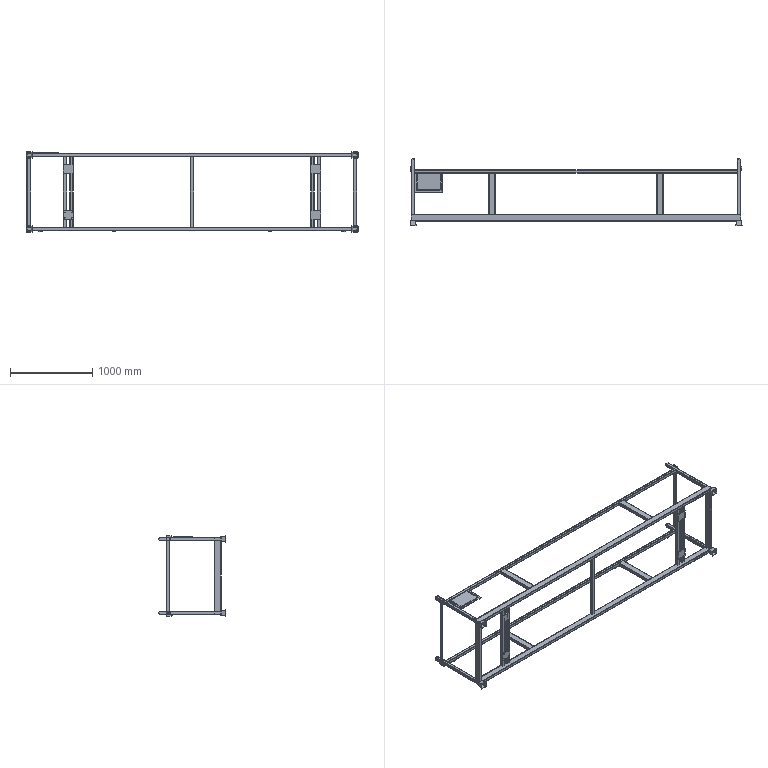Part | SolidWorks | features ReferencePattern 11, MirrorCompFeat 6, LocalLPattern 2 | 68 solids | 924 faces | box 4036 x 824.161 x 980 mm | volume 15514087 mm3 | plane 578 | cylinder 314 | sphere 32 | commonest cylinder face diameters 6 x128 12 x84 10 x36 1 x32 8.5 x16 1.473 x9